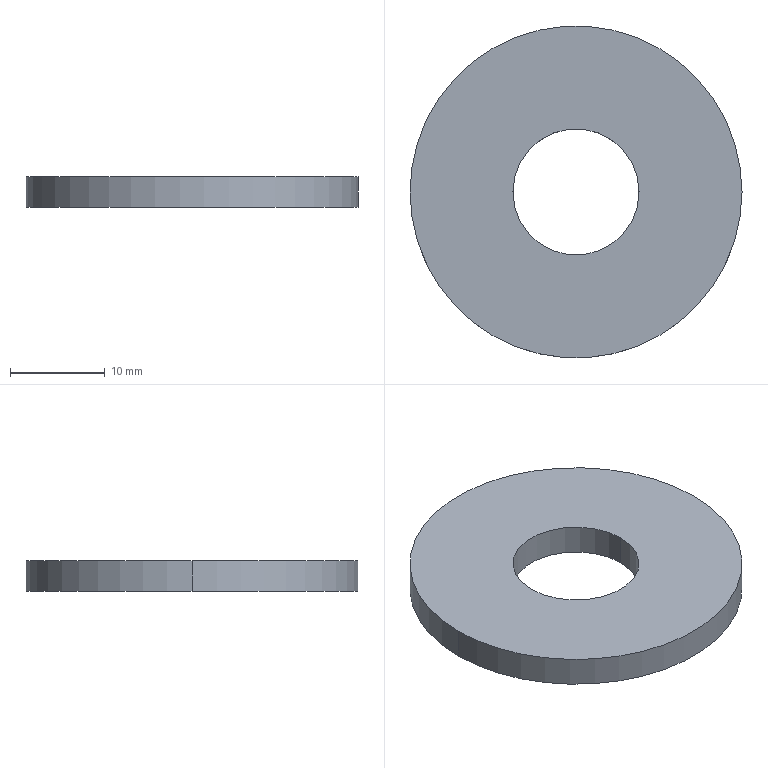Part | SolidWorks | features FlatPattern 1, SMBaseFlange 1, SheetMetal 1 | 1 solid | 6 faces | box 35 x 35 x 3.2 mm | volume 2634 mm3 | cylinder 4 | plane 2 | commonest cylinder face diameters 13.3 x2 35 x2
STEP:
#1=CARTESIAN_POINT('',(-119.104,88.65,3.2));
#2=VERTEX_POINT('',#1);
#3=CARTESIAN_POINT('',(-105.804,88.65,3.2));
#4=VERTEX_POINT('',#3);
#5=CARTESIAN_POINT('',(-112.454,88.65,3.2));
#6=DIRECTION('',(0.,0.,1.));
#7=DIRECTION('',(1.,0.,0.));
#8=AXIS2_PLACEMENT_3D('',#5,#6,#7);
#9=CIRCLE('',#8,6.65);
#10=EDGE_CURVE('',#2,#4,#9,.T.);
#11=ORIENTED_EDGE('',*,*,#10,.T.);
#12=CARTESIAN_POINT('',(-105.804,88.65,0.));
#13=VERTEX_POINT('',#12);
#14=CARTESIAN_POINT('',(-105.804,88.65,3.2));
#15=DIRECTION('',(0.,0.,-1.));
#16=VECTOR('',#15,1000.);
#17=LINE('',#14,#16);
#18=EDGE_CURVE('',#4,#13,#17,.T.);
#19=ORIENTED_EDGE('',*,*,#18,.T.);
#20=CARTESIAN_POINT('',(-119.104,88.65,0.));
#21=VERTEX_POINT('',#20);
#22=CARTESIAN_POINT('',(-112.454,88.65,0.));
#23=DIRECTION('',(0.,0.,1.));
#24=DIRECTION('',(1.,0.,0.));
#25=AXIS2_PLACEMENT_3D('',#22,#23,#24);
#26=CIRCLE('',#25,6.65);
#27=EDGE_CURVE('',#21,#13,#26,.T.);
#28=ORIENTED_EDGE('',*,*,#27,.F.);
#29=CARTESIAN_POINT('',(-119.104,88.65,3.2));
#30=DIRECTION('',(0.,0.,-1.));
#31=VECTOR('',#30,1000.);
#32=LINE('',#29,#31);
#33=EDGE_CURVE('',#2,#21,#32,.T.);
#34=ORIENTED_EDGE('',*,*,#33,.F.);
#35=EDGE_LOOP('',(#11,#19,#28,#34));
#36=FACE_OUTER_BOUND('',#35,.T.);
#37=CARTESIAN_POINT('',(-112.454,88.65,3.2));
#38=DIRECTION('',(0.,0.,-1.));
#39=DIRECTION('',(-1.,0.,0.));
#40=AXIS2_PLACEMENT_3D('',#37,#38,#39);
#41=CYLINDRICAL_SURFACE('',#40,6.65);
#42=ADVANCED_FACE('',(#36),#41,.F.);
#43=CARTESIAN_POINT('',(-94.954,88.65,3.2));
#44=VERTEX_POINT('',#43);
#45=CARTESIAN_POINT('',(-129.954,88.65,3.2));
#46=VERTEX_POINT('',#45);
#47=CARTESIAN_POINT('',(-112.454,88.65,3.2));
#48=DIRECTION('',(0.,0.,1.));
#49=DIRECTION('',(1.,0.,0.));
#50=AXIS2_PLACEMENT_3D('',#47,#48,#49);
#51=CIRCLE('',#50,17.5);
#52=EDGE_CURVE('',#44,#46,#51,.T.);
#53=ORIENTED_EDGE('',*,*,#52,.F.);
#54=CARTESIAN_POINT('',(-94.954,88.65,0.));
#55=VERTEX_POINT('',#54);
#56=CARTESIAN_POINT('',(-94.954,88.65,3.2));
#57=DIRECTION('',(0.,0.,-1.));
#58=VECTOR('',#57,1000.);
#59=LINE('',#56,#58);
#60=EDGE_CURVE('',#44,#55,#59,.T.);
#61=ORIENTED_EDGE('',*,*,#60,.T.);
#62=CARTESIAN_POINT('',(-129.954,88.65,0.));
#63=VERTEX_POINT('',#62);
#64=CARTESIAN_POINT('',(-112.454,88.65,0.));
#65=DIRECTION('',(0.,0.,1.));
#66=DIRECTION('',(1.,0.,0.));
#67=AXIS2_PLACEMENT_3D('',#64,#65,#66);
#68=CIRCLE('',#67,17.5);
#69=EDGE_CURVE('',#55,#63,#68,.T.);
#70=ORIENTED_EDGE('',*,*,#69,.T.);
#71=CARTESIAN_POINT('',(-129.954,88.65,3.2));
#72=DIRECTION('',(0.,0.,-1.));
#73=VECTOR('',#72,1000.);
#74=LINE('',#71,#73);
#75=EDGE_CURVE('',#46,#63,#74,.T.);
#76=ORIENTED_EDGE('',*,*,#75,.F.);
#77=EDGE_LOOP('',(#53,#61,#70,#76));
#78=FACE_OUTER_BOUND('',#77,.T.);
#79=CARTESIAN_POINT('',(-112.454,88.65,3.2));
#80=DIRECTION('',(0.,0.,-1.));
#81=DIRECTION('',(-1.,0.,0.));
#82=AXIS2_PLACEMENT_3D('',#79,#80,#81);
#83=CYLINDRICAL_SURFACE('',#82,17.5);
#84=ADVANCED_FACE('',(#78),#83,.T.);
#85=CARTESIAN_POINT('',(-112.454,88.65,3.2));
#86=DIRECTION('',(0.,0.,1.));
#87=DIRECTION('',(1.,0.,0.));
#88=AXIS2_PLACEMENT_3D('',#85,#86,#87);
#89=CIRCLE('',#88,17.5);
#90=EDGE_CURVE('',#46,#44,#89,.T.);
#91=ORIENTED_EDGE('',*,*,#90,.T.);
#92=ORIENTED_EDGE('',*,*,#52,.T.);
#93=EDGE_LOOP('',(#91,#92));
#94=FACE_OUTER_BOUND('',#93,.T.);
#95=ORIENTED_EDGE('',*,*,#10,.F.);
#96=CARTESIAN_POINT('',(-112.454,88.65,3.2));
#97=DIRECTION('',(0.,0.,1.));
#98=DIRECTION('',(1.,0.,0.));
#99=AXIS2_PLACEMENT_3D('',#96,#97,#98);
#100=CIRCLE('',#99,6.65);
#101=EDGE_CURVE('',#4,#2,#100,.T.);
#102=ORIENTED_EDGE('',*,*,#101,.F.);
#103=EDGE_LOOP('',(#95,#102));
#104=FACE_BOUND('',#103,.T.);
#105=CARTESIAN_POINT('',(-112.454,88.65,3.2));
#106=DIRECTION('',(0.,0.,1.));
#107=DIRECTION('',(1.,0.,0.));
#108=AXIS2_PLACEMENT_3D('',#105,#106,#107);
#109=PLANE('',#108);
#110=ADVANCED_FACE('',(#94,#104),#109,.T.);
#111=CARTESIAN_POINT('',(-112.454,88.65,0.));
#112=DIRECTION('',(0.,0.,1.));
#113=DIRECTION('',(1.,0.,0.));
#114=AXIS2_PLACEMENT_3D('',#111,#112,#113);
#115=CIRCLE('',#114,17.5);
#116=EDGE_CURVE('',#63,#55,#115,.T.);
#117=ORIENTED_EDGE('',*,*,#116,.F.);
#118=ORIENTED_EDGE('',*,*,#69,.F.);
#119=EDGE_LOOP('',(#117,#118));
#120=FACE_OUTER_BOUND('',#119,.T.);
#121=ORIENTED_EDGE('',*,*,#27,.T.);
#122=CARTESIAN_POINT('',(-112.454,88.65,0.));
#123=DIRECTION('',(0.,0.,1.));
#124=DIRECTION('',(1.,0.,0.));
#125=AXIS2_PLACEMENT_3D('',#122,#123,#124);
#126=CIRCLE('',#125,6.65);
#127=EDGE_CURVE('',#13,#21,#126,.T.);
#128=ORIENTED_EDGE('',*,*,#127,.T.);
#129=EDGE_LOOP('',(#121,#128));
#130=FACE_BOUND('',#129,.T.);
#131=CARTESIAN_POINT('',(-112.454,88.65,0.));
#132=DIRECTION('',(0.,0.,1.));
#133=DIRECTION('',(1.,0.,0.));
#134=AXIS2_PLACEMENT_3D('',#131,#132,#133);
#135=PLANE('',#134);
#136=ADVANCED_FACE('',(#120,#130),#135,.F.);
#137=ORIENTED_EDGE('',*,*,#60,.F.);
#138=ORIENTED_EDGE('',*,*,#90,.F.);
#139=ORIENTED_EDGE('',*,*,#75,.T.);
#140=ORIENTED_EDGE('',*,*,#116,.T.);
#141=EDGE_LOOP('',(#137,#138,#139,#140));
#142=FACE_OUTER_BOUND('',#141,.T.);
#143=CARTESIAN_POINT('',(-112.454,88.65,3.2));
#144=DIRECTION('',(0.,0.,-1.));
#145=DIRECTION('',(-1.,0.,0.));
#146=AXIS2_PLACEMENT_3D('',#143,#144,#145);
#147=CYLINDRICAL_SURFACE('',#146,17.5);
#148=ADVANCED_FACE('',(#142),#147,.T.);
#149=ORIENTED_EDGE('',*,*,#18,.F.);
#150=ORIENTED_EDGE('',*,*,#101,.T.);
#151=ORIENTED_EDGE('',*,*,#33,.T.);
#152=ORIENTED_EDGE('',*,*,#127,.F.);
#153=EDGE_LOOP('',(#149,#150,#151,#152));
#154=FACE_OUTER_BOUND('',#153,.T.);
#155=CARTESIAN_POINT('',(-112.454,88.65,3.2));
#156=DIRECTION('',(0.,0.,-1.));
#157=DIRECTION('',(-1.,0.,0.));
#158=AXIS2_PLACEMENT_3D('',#155,#156,#157);
#159=CYLINDRICAL_SURFACE('',#158,6.65);
#160=ADVANCED_FACE('',(#154),#159,.F.);
#161=CLOSED_SHELL('',(#42,#84,#110,#136,#148,#160));
#162=MANIFOLD_SOLID_BREP('',#161);
#163=CARTESIAN_POINT('',(0.,0.,0.));
#164=DIRECTION('',(0.,0.,1.));
#165=DIRECTION('',(1.,0.,0.));
#166=AXIS2_PLACEMENT_3D('',#163,#164,#165);
#167=(LENGTH_UNIT()NAMED_UNIT(*)SI_UNIT(.MILLI.,.METRE.));
#168=UNCERTAINTY_MEASURE_WITH_UNIT(LENGTH_MEASURE(0.00001),#167,'','');
#169=(NAMED_UNIT(*)PLANE_ANGLE_UNIT()SI_UNIT($,.RADIAN.));
#170=(NAMED_UNIT(*)SI_UNIT($,.STERADIAN.)SOLID_ANGLE_UNIT());
#171=(GEOMETRIC_REPRESENTATION_CONTEXT(3)GLOBAL_UNCERTAINTY_ASSIGNED_CONTEXT((#168))GLOBAL_UNIT_ASSIGNED_CONTEXT((#167,#169,#170))REPRESENTATION_CONTEXT('',''));
#172=ADVANCED_BREP_SHAPE_REPRESENTATION('',(#162,#166),#171);